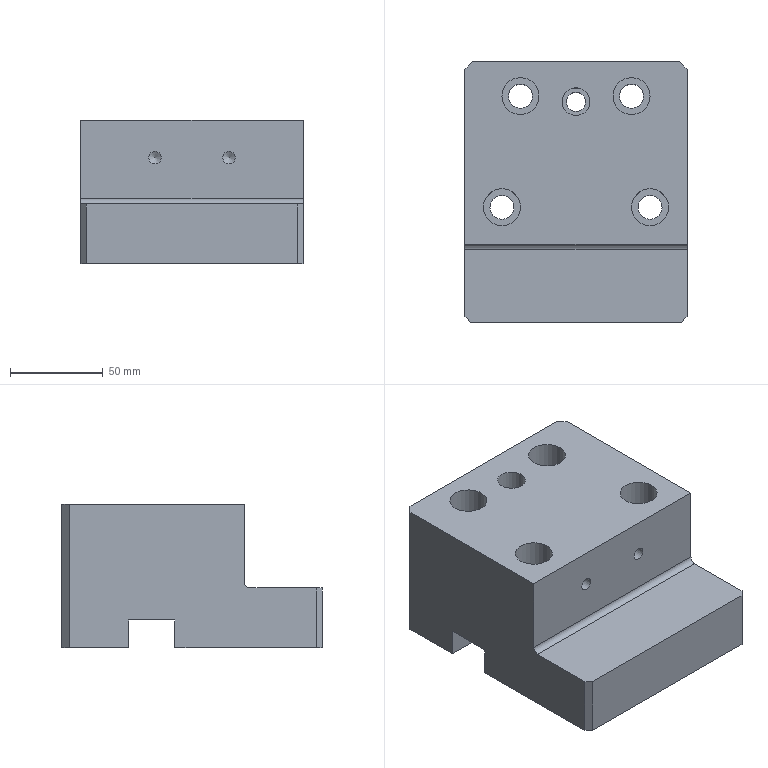Part | STEP file | 1_id1582_x_t | 1 solid | 42 faces | box 120 x 140.586 x 77.52 mm | volume 963070 mm3 | plane 21 | cylinder 15 | cone 6 | commonest cylinder face diameters 13 x4 20 x4 6.75 x2 7.938 x2 6 x1 10.25 x1